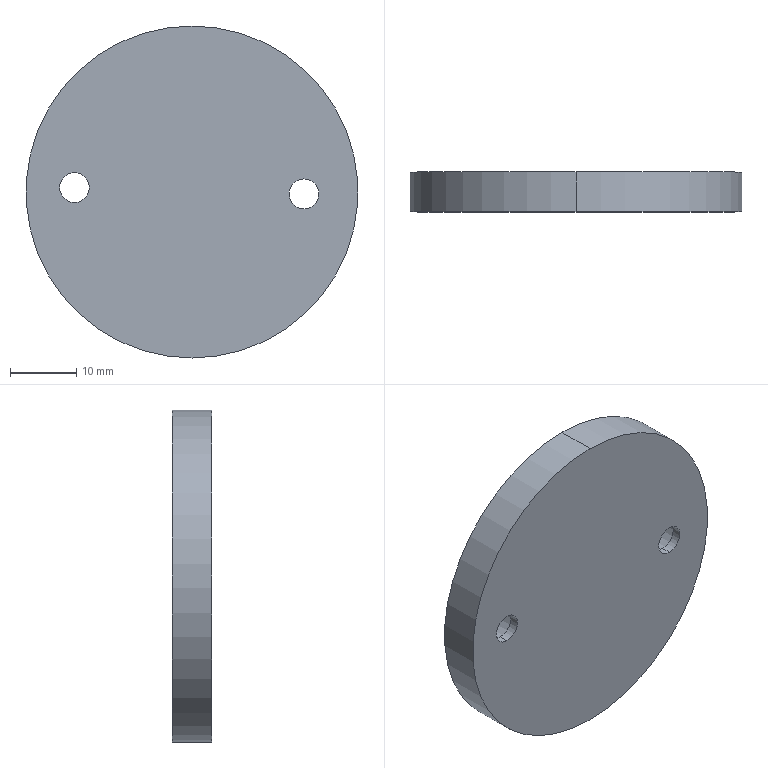Part | SolidWorks | features 3DProfileFeature 1, Extrusion 1, HoleWzd 1 | 1 solid | 14 faces | box 50 x 6 x 50 mm | volume 11274 mm3 | cylinder 10 | plane 4 | commonest cylinder face diameters 4.5 x4 8 x4 50 x2
STEP:
#1=CARTESIAN_POINT('',(16.865,1.4,-4.29));
#2=VERTEX_POINT('',#1);
#3=CARTESIAN_POINT('',(16.865,1.4,3.71));
#4=VERTEX_POINT('',#3);
#5=CARTESIAN_POINT('',(16.865,1.4,-0.2895));
#6=DIRECTION('',(0.,1.,0.));
#7=DIRECTION('',(0.,0.,1.));
#8=AXIS2_PLACEMENT_3D('',#5,#6,#7);
#9=CIRCLE('',#8,4.);
#10=EDGE_CURVE('',#2,#4,#9,.T.);
#11=ORIENTED_EDGE('',*,*,#10,.F.);
#12=CARTESIAN_POINT('',(16.865,6.,-4.29));
#13=VERTEX_POINT('',#12);
#14=CARTESIAN_POINT('',(16.865,6.,-4.29));
#15=DIRECTION('',(0.,1.,0.));
#16=VECTOR('',#15,1000.);
#17=LINE('',#14,#16);
#18=EDGE_CURVE('',#2,#13,#17,.T.);
#19=ORIENTED_EDGE('',*,*,#18,.T.);
#20=CARTESIAN_POINT('',(16.865,6.,3.71));
#21=VERTEX_POINT('',#20);
#22=CARTESIAN_POINT('',(16.865,6.,-0.2895));
#23=DIRECTION('',(0.,1.,0.));
#24=DIRECTION('',(0.,0.,1.));
#25=AXIS2_PLACEMENT_3D('',#22,#23,#24);
#26=CIRCLE('',#25,4.);
#27=EDGE_CURVE('',#13,#21,#26,.T.);
#28=ORIENTED_EDGE('',*,*,#27,.T.);
#29=CARTESIAN_POINT('',(16.865,6.,3.71));
#30=DIRECTION('',(0.,1.,0.));
#31=VECTOR('',#30,1000.);
#32=LINE('',#29,#31);
#33=EDGE_CURVE('',#4,#21,#32,.T.);
#34=ORIENTED_EDGE('',*,*,#33,.F.);
#35=EDGE_LOOP('',(#11,#19,#28,#34));
#36=FACE_OUTER_BOUND('',#35,.T.);
#37=CARTESIAN_POINT('',(16.865,6.,-0.2895));
#38=DIRECTION('',(0.,1.,0.));
#39=DIRECTION('',(0.,0.,1.));
#40=AXIS2_PLACEMENT_3D('',#37,#38,#39);
#41=CYLINDRICAL_SURFACE('',#40,4.);
#42=ADVANCED_FACE('',(#36),#41,.F.);
#43=CARTESIAN_POINT('',(16.865,0.,-2.54));
#44=VERTEX_POINT('',#43);
#45=CARTESIAN_POINT('',(16.865,0.,1.96));
#46=VERTEX_POINT('',#45);
#47=CARTESIAN_POINT('',(16.865,0.,-0.2895));
#48=DIRECTION('',(0.,1.,0.));
#49=DIRECTION('',(0.,0.,1.));
#50=AXIS2_PLACEMENT_3D('',#47,#48,#49);
#51=CIRCLE('',#50,2.25);
#52=EDGE_CURVE('',#44,#46,#51,.T.);
#53=ORIENTED_EDGE('',*,*,#52,.F.);
#54=CARTESIAN_POINT('',(16.865,1.4,-2.54));
#55=VERTEX_POINT('',#54);
#56=CARTESIAN_POINT('',(16.865,6.,-2.54));
#57=DIRECTION('',(0.,1.,0.));
#58=VECTOR('',#57,1000.);
#59=LINE('',#56,#58);
#60=EDGE_CURVE('',#44,#55,#59,.T.);
#61=ORIENTED_EDGE('',*,*,#60,.T.);
#62=CARTESIAN_POINT('',(16.865,1.4,1.96));
#63=VERTEX_POINT('',#62);
#64=CARTESIAN_POINT('',(16.865,1.4,-0.2895));
#65=DIRECTION('',(0.,1.,0.));
#66=DIRECTION('',(0.,0.,1.));
#67=AXIS2_PLACEMENT_3D('',#64,#65,#66);
#68=CIRCLE('',#67,2.25);
#69=EDGE_CURVE('',#55,#63,#68,.T.);
#70=ORIENTED_EDGE('',*,*,#69,.T.);
#71=CARTESIAN_POINT('',(16.865,6.,1.96));
#72=DIRECTION('',(0.,1.,0.));
#73=VECTOR('',#72,1000.);
#74=LINE('',#71,#73);
#75=EDGE_CURVE('',#46,#63,#74,.T.);
#76=ORIENTED_EDGE('',*,*,#75,.F.);
#77=EDGE_LOOP('',(#53,#61,#70,#76));
#78=FACE_OUTER_BOUND('',#77,.T.);
#79=CARTESIAN_POINT('',(16.865,6.,-0.2895));
#80=DIRECTION('',(0.,1.,0.));
#81=DIRECTION('',(0.,0.,1.));
#82=AXIS2_PLACEMENT_3D('',#79,#80,#81);
#83=CYLINDRICAL_SURFACE('',#82,2.25);
#84=ADVANCED_FACE('',(#78),#83,.F.);
#85=CARTESIAN_POINT('',(-17.703,1.4,-3.328));
#86=VERTEX_POINT('',#85);
#87=CARTESIAN_POINT('',(-17.703,1.4,4.672));
#88=VERTEX_POINT('',#87);
#89=CARTESIAN_POINT('',(-17.703,1.4,0.6722));
#90=DIRECTION('',(0.,1.,0.));
#91=DIRECTION('',(0.,0.,1.));
#92=AXIS2_PLACEMENT_3D('',#89,#90,#91);
#93=CIRCLE('',#92,4.);
#94=EDGE_CURVE('',#86,#88,#93,.T.);
#95=ORIENTED_EDGE('',*,*,#94,.F.);
#96=CARTESIAN_POINT('',(-17.703,6.,-3.328));
#97=VERTEX_POINT('',#96);
#98=CARTESIAN_POINT('',(-17.703,6.,-3.328));
#99=DIRECTION('',(0.,1.,0.));
#100=VECTOR('',#99,1000.);
#101=LINE('',#98,#100);
#102=EDGE_CURVE('',#86,#97,#101,.T.);
#103=ORIENTED_EDGE('',*,*,#102,.T.);
#104=CARTESIAN_POINT('',(-17.703,6.,4.672));
#105=VERTEX_POINT('',#104);
#106=CARTESIAN_POINT('',(-17.703,6.,0.6722));
#107=DIRECTION('',(0.,1.,0.));
#108=DIRECTION('',(0.,0.,1.));
#109=AXIS2_PLACEMENT_3D('',#106,#107,#108);
#110=CIRCLE('',#109,4.);
#111=EDGE_CURVE('',#97,#105,#110,.T.);
#112=ORIENTED_EDGE('',*,*,#111,.T.);
#113=CARTESIAN_POINT('',(-17.703,6.,4.672));
#114=DIRECTION('',(0.,1.,0.));
#115=VECTOR('',#114,1000.);
#116=LINE('',#113,#115);
#117=EDGE_CURVE('',#88,#105,#116,.T.);
#118=ORIENTED_EDGE('',*,*,#117,.F.);
#119=EDGE_LOOP('',(#95,#103,#112,#118));
#120=FACE_OUTER_BOUND('',#119,.T.);
#121=CARTESIAN_POINT('',(-17.703,6.,0.6722));
#122=DIRECTION('',(0.,1.,0.));
#123=DIRECTION('',(0.,0.,1.));
#124=AXIS2_PLACEMENT_3D('',#121,#122,#123);
#125=CYLINDRICAL_SURFACE('',#124,4.);
#126=ADVANCED_FACE('',(#120),#125,.F.);
#127=CARTESIAN_POINT('',(-17.703,0.,-1.578));
#128=VERTEX_POINT('',#127);
#129=CARTESIAN_POINT('',(-17.703,0.,2.922));
#130=VERTEX_POINT('',#129);
#131=CARTESIAN_POINT('',(-17.703,0.,0.6722));
#132=DIRECTION('',(0.,1.,0.));
#133=DIRECTION('',(0.,0.,1.));
#134=AXIS2_PLACEMENT_3D('',#131,#132,#133);
#135=CIRCLE('',#134,2.25);
#136=EDGE_CURVE('',#128,#130,#135,.T.);
#137=ORIENTED_EDGE('',*,*,#136,.F.);
#138=CARTESIAN_POINT('',(-17.703,1.4,-1.578));
#139=VERTEX_POINT('',#138);
#140=CARTESIAN_POINT('',(-17.703,6.,-1.578));
#141=DIRECTION('',(0.,1.,0.));
#142=VECTOR('',#141,1000.);
#143=LINE('',#140,#142);
#144=EDGE_CURVE('',#128,#139,#143,.T.);
#145=ORIENTED_EDGE('',*,*,#144,.T.);
#146=CARTESIAN_POINT('',(-17.703,1.4,2.922));
#147=VERTEX_POINT('',#146);
#148=CARTESIAN_POINT('',(-17.703,1.4,0.6722));
#149=DIRECTION('',(0.,1.,0.));
#150=DIRECTION('',(0.,0.,1.));
#151=AXIS2_PLACEMENT_3D('',#148,#149,#150);
#152=CIRCLE('',#151,2.25);
#153=EDGE_CURVE('',#139,#147,#152,.T.);
#154=ORIENTED_EDGE('',*,*,#153,.T.);
#155=CARTESIAN_POINT('',(-17.703,6.,2.922));
#156=DIRECTION('',(0.,1.,0.));
#157=VECTOR('',#156,1000.);
#158=LINE('',#155,#157);
#159=EDGE_CURVE('',#130,#147,#158,.T.);
#160=ORIENTED_EDGE('',*,*,#159,.F.);
#161=EDGE_LOOP('',(#137,#145,#154,#160));
#162=FACE_OUTER_BOUND('',#161,.T.);
#163=CARTESIAN_POINT('',(-17.703,6.,0.6722));
#164=DIRECTION('',(0.,1.,0.));
#165=DIRECTION('',(0.,0.,1.));
#166=AXIS2_PLACEMENT_3D('',#163,#164,#165);
#167=CYLINDRICAL_SURFACE('',#166,2.25);
#168=ADVANCED_FACE('',(#162),#167,.F.);
#169=CARTESIAN_POINT('',(0.,6.,25.));
#170=VERTEX_POINT('',#169);
#171=CARTESIAN_POINT('',(0.,6.,-25.));
#172=VERTEX_POINT('',#171);
#173=CARTESIAN_POINT('',(0.,6.,0.));
#174=DIRECTION('',(0.,1.,0.));
#175=DIRECTION('',(0.,0.,1.));
#176=AXIS2_PLACEMENT_3D('',#173,#174,#175);
#177=CIRCLE('',#176,25.);
#178=EDGE_CURVE('',#170,#172,#177,.T.);
#179=ORIENTED_EDGE('',*,*,#178,.F.);
#180=CARTESIAN_POINT('',(0.,0.,25.));
#181=VERTEX_POINT('',#180);
#182=CARTESIAN_POINT('',(0.,6.,25.));
#183=DIRECTION('',(0.,-1.,0.));
#184=VECTOR('',#183,1000.);
#185=LINE('',#182,#184);
#186=EDGE_CURVE('',#170,#181,#185,.T.);
#187=ORIENTED_EDGE('',*,*,#186,.T.);
#188=CARTESIAN_POINT('',(0.,0.,-25.));
#189=VERTEX_POINT('',#188);
#190=CARTESIAN_POINT('',(0.,0.,0.));
#191=DIRECTION('',(0.,1.,0.));
#192=DIRECTION('',(0.,0.,1.));
#193=AXIS2_PLACEMENT_3D('',#190,#191,#192);
#194=CIRCLE('',#193,25.);
#195=EDGE_CURVE('',#181,#189,#194,.T.);
#196=ORIENTED_EDGE('',*,*,#195,.T.);
#197=CARTESIAN_POINT('',(0.,6.,-25.));
#198=DIRECTION('',(0.,-1.,0.));
#199=VECTOR('',#198,1000.);
#200=LINE('',#197,#199);
#201=EDGE_CURVE('',#172,#189,#200,.T.);
#202=ORIENTED_EDGE('',*,*,#201,.F.);
#203=EDGE_LOOP('',(#179,#187,#196,#202));
#204=FACE_OUTER_BOUND('',#203,.T.);
#205=CARTESIAN_POINT('',(0.,6.,0.));
#206=DIRECTION('',(0.,-1.,0.));
#207=DIRECTION('',(0.,0.,-1.));
#208=AXIS2_PLACEMENT_3D('',#205,#206,#207);
#209=CYLINDRICAL_SURFACE('',#208,25.);
#210=ADVANCED_FACE('',(#204),#209,.T.);
#211=ORIENTED_EDGE('',*,*,#186,.F.);
#212=CARTESIAN_POINT('',(0.,6.,0.));
#213=DIRECTION('',(0.,1.,0.));
#214=DIRECTION('',(0.,0.,1.));
#215=AXIS2_PLACEMENT_3D('',#212,#213,#214);
#216=CIRCLE('',#215,25.);
#217=EDGE_CURVE('',#172,#170,#216,.T.);
#218=ORIENTED_EDGE('',*,*,#217,.F.);
#219=ORIENTED_EDGE('',*,*,#201,.T.);
#220=CARTESIAN_POINT('',(0.,0.,0.));
#221=DIRECTION('',(0.,1.,0.));
#222=DIRECTION('',(0.,0.,1.));
#223=AXIS2_PLACEMENT_3D('',#220,#221,#222);
#224=CIRCLE('',#223,25.);
#225=EDGE_CURVE('',#189,#181,#224,.T.);
#226=ORIENTED_EDGE('',*,*,#225,.T.);
#227=EDGE_LOOP('',(#211,#218,#219,#226));
#228=FACE_OUTER_BOUND('',#227,.T.);
#229=CARTESIAN_POINT('',(0.,6.,0.));
#230=DIRECTION('',(0.,-1.,0.));
#231=DIRECTION('',(0.,0.,-1.));
#232=AXIS2_PLACEMENT_3D('',#229,#230,#231);
#233=CYLINDRICAL_SURFACE('',#232,25.);
#234=ADVANCED_FACE('',(#228),#233,.T.);
#235=CARTESIAN_POINT('',(16.865,6.,-0.2895));
#236=DIRECTION('',(0.,1.,0.));
#237=DIRECTION('',(0.,0.,1.));
#238=AXIS2_PLACEMENT_3D('',#235,#236,#237);
#239=CIRCLE('',#238,4.);
#240=EDGE_CURVE('',#21,#13,#239,.T.);
#241=ORIENTED_EDGE('',*,*,#240,.F.);
#242=ORIENTED_EDGE('',*,*,#27,.F.);
#243=EDGE_LOOP('',(#241,#242));
#244=FACE_BOUND('',#243,.T.);
#245=CARTESIAN_POINT('',(-17.703,6.,0.6722));
#246=DIRECTION('',(0.,1.,0.));
#247=DIRECTION('',(0.,0.,1.));
#248=AXIS2_PLACEMENT_3D('',#245,#246,#247);
#249=CIRCLE('',#248,4.);
#250=EDGE_CURVE('',#105,#97,#249,.T.);
#251=ORIENTED_EDGE('',*,*,#250,.F.);
#252=ORIENTED_EDGE('',*,*,#111,.F.);
#253=EDGE_LOOP('',(#251,#252));
#254=FACE_BOUND('',#253,.T.);
#255=ORIENTED_EDGE('',*,*,#217,.T.);
#256=ORIENTED_EDGE('',*,*,#178,.T.);
#257=EDGE_LOOP('',(#255,#256));
#258=FACE_OUTER_BOUND('',#257,.T.);
#259=CARTESIAN_POINT('',(0.,6.,0.));
#260=DIRECTION('',(0.,1.,0.));
#261=DIRECTION('',(0.,0.,1.));
#262=AXIS2_PLACEMENT_3D('',#259,#260,#261);
#263=PLANE('',#262);
#264=ADVANCED_FACE('',(#244,#254,#258),#263,.T.);
#265=CARTESIAN_POINT('',(16.865,0.,-0.2895));
#266=DIRECTION('',(0.,1.,0.));
#267=DIRECTION('',(0.,0.,1.));
#268=AXIS2_PLACEMENT_3D('',#265,#266,#267);
#269=CIRCLE('',#268,2.25);
#270=EDGE_CURVE('',#46,#44,#269,.T.);
#271=ORIENTED_EDGE('',*,*,#270,.T.);
#272=ORIENTED_EDGE('',*,*,#52,.T.);
#273=EDGE_LOOP('',(#271,#272));
#274=FACE_BOUND('',#273,.T.);
#275=CARTESIAN_POINT('',(-17.703,0.,0.6722));
#276=DIRECTION('',(0.,1.,0.));
#277=DIRECTION('',(0.,0.,1.));
#278=AXIS2_PLACEMENT_3D('',#275,#276,#277);
#279=CIRCLE('',#278,2.25);
#280=EDGE_CURVE('',#130,#128,#279,.T.);
#281=ORIENTED_EDGE('',*,*,#280,.T.);
#282=ORIENTED_EDGE('',*,*,#136,.T.);
#283=EDGE_LOOP('',(#281,#282));
#284=FACE_BOUND('',#283,.T.);
#285=ORIENTED_EDGE('',*,*,#225,.F.);
#286=ORIENTED_EDGE('',*,*,#195,.F.);
#287=EDGE_LOOP('',(#285,#286));
#288=FACE_OUTER_BOUND('',#287,.T.);
#289=CARTESIAN_POINT('',(0.,0.,0.));
#290=DIRECTION('',(0.,1.,0.));
#291=DIRECTION('',(0.,0.,1.));
#292=AXIS2_PLACEMENT_3D('',#289,#290,#291);
#293=PLANE('',#292);
#294=ADVANCED_FACE('',(#274,#284,#288),#293,.F.);
#295=ORIENTED_EDGE('',*,*,#144,.F.);
#296=ORIENTED_EDGE('',*,*,#280,.F.);
#297=ORIENTED_EDGE('',*,*,#159,.T.);
#298=CARTESIAN_POINT('',(-17.703,1.4,0.6722));
#299=DIRECTION('',(0.,1.,0.));
#300=DIRECTION('',(0.,0.,1.));
#301=AXIS2_PLACEMENT_3D('',#298,#299,#300);
#302=CIRCLE('',#301,2.25);
#303=EDGE_CURVE('',#147,#139,#302,.T.);
#304=ORIENTED_EDGE('',*,*,#303,.T.);
#305=EDGE_LOOP('',(#295,#296,#297,#304));
#306=FACE_OUTER_BOUND('',#305,.T.);
#307=CARTESIAN_POINT('',(-17.703,6.,0.6722));
#308=DIRECTION('',(0.,1.,0.));
#309=DIRECTION('',(0.,0.,1.));
#310=AXIS2_PLACEMENT_3D('',#307,#308,#309);
#311=CYLINDRICAL_SURFACE('',#310,2.25);
#312=ADVANCED_FACE('',(#306),#311,.F.);
#313=ORIENTED_EDGE('',*,*,#303,.F.);
#314=ORIENTED_EDGE('',*,*,#153,.F.);
#315=EDGE_LOOP('',(#313,#314));
#316=FACE_BOUND('',#315,.T.);
#317=CARTESIAN_POINT('',(-17.703,1.4,0.6722));
#318=DIRECTION('',(0.,1.,0.));
#319=DIRECTION('',(0.,0.,1.));
#320=AXIS2_PLACEMENT_3D('',#317,#318,#319);
#321=CIRCLE('',#320,4.);
#322=EDGE_CURVE('',#88,#86,#321,.T.);
#323=ORIENTED_EDGE('',*,*,#322,.T.);
#324=ORIENTED_EDGE('',*,*,#94,.T.);
#325=EDGE_LOOP('',(#323,#324));
#326=FACE_OUTER_BOUND('',#325,.T.);
#327=CARTESIAN_POINT('',(-15.453,1.4,0.6722));
#328=DIRECTION('',(0.,-1.,0.));
#329=DIRECTION('',(0.,0.,-1.));
#330=AXIS2_PLACEMENT_3D('',#327,#328,#329);
#331=PLANE('',#330);
#332=ADVANCED_FACE('',(#316,#326),#331,.F.);
#333=ORIENTED_EDGE('',*,*,#102,.F.);
#334=ORIENTED_EDGE('',*,*,#322,.F.);
#335=ORIENTED_EDGE('',*,*,#117,.T.);
#336=ORIENTED_EDGE('',*,*,#250,.T.);
#337=EDGE_LOOP('',(#333,#334,#335,#336));
#338=FACE_OUTER_BOUND('',#337,.T.);
#339=CARTESIAN_POINT('',(-17.703,6.,0.6722));
#340=DIRECTION('',(0.,1.,0.));
#341=DIRECTION('',(0.,0.,1.));
#342=AXIS2_PLACEMENT_3D('',#339,#340,#341);
#343=CYLINDRICAL_SURFACE('',#342,4.);
#344=ADVANCED_FACE('',(#338),#343,.F.);
#345=ORIENTED_EDGE('',*,*,#60,.F.);
#346=ORIENTED_EDGE('',*,*,#270,.F.);
#347=ORIENTED_EDGE('',*,*,#75,.T.);
#348=CARTESIAN_POINT('',(16.865,1.4,-0.2895));
#349=DIRECTION('',(0.,1.,0.));
#350=DIRECTION('',(0.,0.,1.));
#351=AXIS2_PLACEMENT_3D('',#348,#349,#350);
#352=CIRCLE('',#351,2.25);
#353=EDGE_CURVE('',#63,#55,#352,.T.);
#354=ORIENTED_EDGE('',*,*,#353,.T.);
#355=EDGE_LOOP('',(#345,#346,#347,#354));
#356=FACE_OUTER_BOUND('',#355,.T.);
#357=CARTESIAN_POINT('',(16.865,6.,-0.2895));
#358=DIRECTION('',(0.,1.,0.));
#359=DIRECTION('',(0.,0.,1.));
#360=AXIS2_PLACEMENT_3D('',#357,#358,#359);
#361=CYLINDRICAL_SURFACE('',#360,2.25);
#362=ADVANCED_FACE('',(#356),#361,.F.);
#363=ORIENTED_EDGE('',*,*,#353,.F.);
#364=ORIENTED_EDGE('',*,*,#69,.F.);
#365=EDGE_LOOP('',(#363,#364));
#366=FACE_BOUND('',#365,.T.);
#367=CARTESIAN_POINT('',(16.865,1.4,-0.2895));
#368=DIRECTION('',(0.,1.,0.));
#369=DIRECTION('',(0.,0.,1.));
#370=AXIS2_PLACEMENT_3D('',#367,#368,#369);
#371=CIRCLE('',#370,4.);
#372=EDGE_CURVE('',#4,#2,#371,.T.);
#373=ORIENTED_EDGE('',*,*,#372,.T.);
#374=ORIENTED_EDGE('',*,*,#10,.T.);
#375=EDGE_LOOP('',(#373,#374));
#376=FACE_OUTER_BOUND('',#375,.T.);
#377=CARTESIAN_POINT('',(19.115,1.4,-0.2895));
#378=DIRECTION('',(0.,-1.,0.));
#379=DIRECTION('',(0.,0.,-1.));
#380=AXIS2_PLACEMENT_3D('',#377,#378,#379);
#381=PLANE('',#380);
#382=ADVANCED_FACE('',(#366,#376),#381,.F.);
#383=ORIENTED_EDGE('',*,*,#18,.F.);
#384=ORIENTED_EDGE('',*,*,#372,.F.);
#385=ORIENTED_EDGE('',*,*,#33,.T.);
#386=ORIENTED_EDGE('',*,*,#240,.T.);
#387=EDGE_LOOP('',(#383,#384,#385,#386));
#388=FACE_OUTER_BOUND('',#387,.T.);
#389=CARTESIAN_POINT('',(16.865,6.,-0.2895));
#390=DIRECTION('',(0.,1.,0.));
#391=DIRECTION('',(0.,0.,1.));
#392=AXIS2_PLACEMENT_3D('',#389,#390,#391);
#393=CYLINDRICAL_SURFACE('',#392,4.);
#394=ADVANCED_FACE('',(#388),#393,.F.);
#395=CLOSED_SHELL('',(#42,#84,#126,#168,#210,#234,#264,#294,#312,#332,#344,#362,#382,#394));
#396=MANIFOLD_SOLID_BREP('',#395);
#397=CARTESIAN_POINT('',(0.,0.,0.));
#398=DIRECTION('',(0.,0.,1.));
#399=DIRECTION('',(1.,0.,0.));
#400=AXIS2_PLACEMENT_3D('',#397,#398,#399);
#401=(LENGTH_UNIT()NAMED_UNIT(*)SI_UNIT(.MILLI.,.METRE.));
#402=UNCERTAINTY_MEASURE_WITH_UNIT(LENGTH_MEASURE(0.00001),#401,'','');
#403=(NAMED_UNIT(*)PLANE_ANGLE_UNIT()SI_UNIT($,.RADIAN.));
#404=(NAMED_UNIT(*)SI_UNIT($,.STERADIAN.)SOLID_ANGLE_UNIT());
#405=(GEOMETRIC_REPRESENTATION_CONTEXT(3)GLOBAL_UNCERTAINTY_ASSIGNED_CONTEXT((#402))GLOBAL_UNIT_ASSIGNED_CONTEXT((#401,#403,#404))REPRESENTATION_CONTEXT('',''));
#406=ADVANCED_BREP_SHAPE_REPRESENTATION('',(#396,#400),#405);